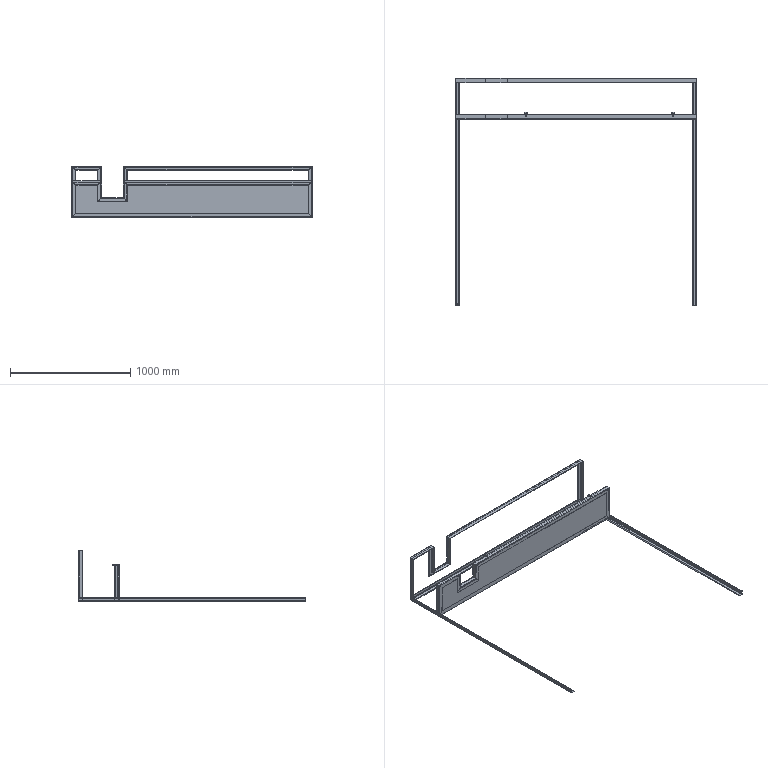Part | SolidWorks | features ICE 6, WeldMemberFeat 3, WeldmentFeature 1 | 20 solids | 212 faces | box 2010 x 1894 x 432 mm | volume 6181114 mm3 | plane 146 | cylinder 66 | commonest cylinder face diameters 10 x56 7 x6 9 x4